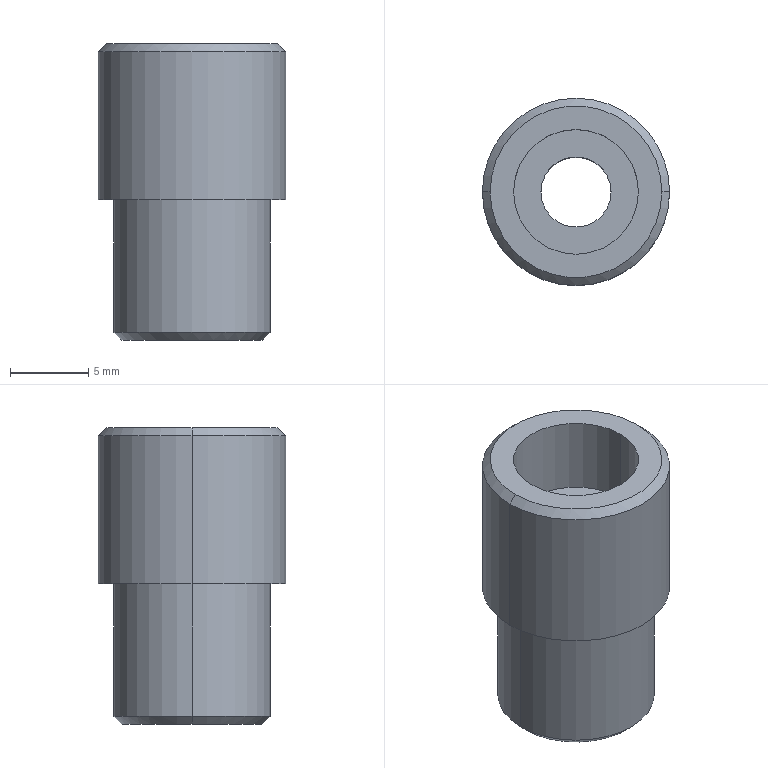Part | STEP file | 227H056246 Shaft_Default | 1 solid | 16 faces | box 12 x 12 x 19 mm | volume 1355 mm3 | cylinder 8 | cone 4 | plane 4 | commonest cylinder face diameters 4.5 x2 8 x2 10 x2 12 x2
STEP:
#1=CARTESIAN_POINT('',(0.,0.,0.));
#2=DIRECTION('',(0.,0.,1.));
#3=DIRECTION('',(1.,0.,0.));
#4=AXIS2_PLACEMENT_3D('',#1,#2,#3);
#5=CARTESIAN_POINT('',(-4.5,0.,-2.));
#6=VERTEX_POINT('',#5);
#7=CARTESIAN_POINT('',(4.5,0.,-2.));
#8=VERTEX_POINT('',#7);
#9=CARTESIAN_POINT('',(0.,0.,-2.));
#10=DIRECTION('',(0.,0.,-1.));
#11=DIRECTION('',(-1.,0.,0.));
#12=AXIS2_PLACEMENT_3D('',#9,#10,#11);
#13=CIRCLE('',#12,4.5);
#14=CARTESIAN_POINT('',(0.,0.,-2.));
#15=DIRECTION('',(0.,0.,1.));
#16=DIRECTION('',(1.,0.,0.));
#17=AXIS2_PLACEMENT_3D('',#14,#15,#16);
#18=CONICAL_SURFACE('',#17,4.5,0.7854);
#19=CARTESIAN_POINT('',(3.142,0.));
#20=DIRECTION('',(-1.,0.));
#21=VECTOR('',#20,1.);
#22=LINE('',#19,#21);
#23=(GEOMETRIC_REPRESENTATION_CONTEXT(2)PARAMETRIC_REPRESENTATION_CONTEXT()REPRESENTATION_CONTEXT('',''));
#24=DEFINITIONAL_REPRESENTATION('',(#22),#23);
#25=PCURVE('',#18,#24);
#26=CARTESIAN_POINT('',(0.,0.,-2.));
#27=DIRECTION('',(0.,0.,-1.));
#28=DIRECTION('',(-1.,0.,0.));
#29=AXIS2_PLACEMENT_3D('',#26,#27,#28);
#30=PLANE('',#29);
#31=CARTESIAN_POINT('',(0.,0.));
#32=DIRECTION('',(1.,0.));
#33=AXIS2_PLACEMENT_2D('',#31,#32);
#34=CIRCLE('',#33,4.5);
#35=(GEOMETRIC_REPRESENTATION_CONTEXT(2)PARAMETRIC_REPRESENTATION_CONTEXT()REPRESENTATION_CONTEXT('',''));
#36=DEFINITIONAL_REPRESENTATION('',(#34),#35);
#37=PCURVE('',#30,#36);
#38=SURFACE_CURVE('',#13,(#25,#37),.PCURVE_S1.);
#39=EDGE_CURVE('',#6,#8,#38,.T.);
#40=ORIENTED_EDGE('',*,*,#39,.F.);
#41=CARTESIAN_POINT('',(-5.,0.,-1.5));
#42=VERTEX_POINT('',#41);
#43=CARTESIAN_POINT('',(-4.5,0.,-2.));
#44=DIRECTION('',(-0.7071,0.,0.7071));
#45=VECTOR('',#44,1.);
#46=LINE('',#43,#45);
#47=CARTESIAN_POINT('',(3.142,0.));
#48=DIRECTION('',(0.,1.));
#49=VECTOR('',#48,1.);
#50=LINE('',#47,#49);
#51=(GEOMETRIC_REPRESENTATION_CONTEXT(2)PARAMETRIC_REPRESENTATION_CONTEXT()REPRESENTATION_CONTEXT('',''));
#52=DEFINITIONAL_REPRESENTATION('',(#50),#51);
#53=PCURVE('',#18,#52);
#54=CARTESIAN_POINT('',(0.,0.,-2.));
#55=DIRECTION('',(0.,0.,1.));
#56=DIRECTION('',(1.,0.,0.));
#57=AXIS2_PLACEMENT_3D('',#54,#55,#56);
#58=CONICAL_SURFACE('',#57,4.5,0.7854);
#59=CARTESIAN_POINT('',(3.142,0.));
#60=DIRECTION('',(0.,1.));
#61=VECTOR('',#60,1.);
#62=LINE('',#59,#61);
#63=(GEOMETRIC_REPRESENTATION_CONTEXT(2)PARAMETRIC_REPRESENTATION_CONTEXT()REPRESENTATION_CONTEXT('',''));
#64=DEFINITIONAL_REPRESENTATION('',(#62),#63);
#65=PCURVE('',#58,#64);
#66=SURFACE_CURVE('',#46,(#53,#65),.PCURVE_S1.);
#67=EDGE_CURVE('',#6,#42,#66,.T.);
#68=ORIENTED_EDGE('',*,*,#67,.T.);
#69=CARTESIAN_POINT('',(5.,0.,-1.5));
#70=VERTEX_POINT('',#69);
#71=CARTESIAN_POINT('',(0.,0.,-1.5));
#72=DIRECTION('',(0.,0.,1.));
#73=DIRECTION('',(-1.,0.,0.));
#74=AXIS2_PLACEMENT_3D('',#71,#72,#73);
#75=CIRCLE('',#74,5.);
#76=CARTESIAN_POINT('',(-3.142,0.5));
#77=DIRECTION('',(1.,0.));
#78=VECTOR('',#77,1.);
#79=LINE('',#76,#78);
#80=(GEOMETRIC_REPRESENTATION_CONTEXT(2)PARAMETRIC_REPRESENTATION_CONTEXT()REPRESENTATION_CONTEXT('',''));
#81=DEFINITIONAL_REPRESENTATION('',(#79),#80);
#82=PCURVE('',#18,#81);
#83=CARTESIAN_POINT('',(0.,0.,12.));
#84=DIRECTION('',(0.,0.,-1.));
#85=DIRECTION('',(-1.,0.,0.));
#86=AXIS2_PLACEMENT_3D('',#83,#84,#85);
#87=CYLINDRICAL_SURFACE('',#86,5.);
#88=CARTESIAN_POINT('',(6.283,13.5));
#89=DIRECTION('',(-1.,0.));
#90=VECTOR('',#89,1.);
#91=LINE('',#88,#90);
#92=(GEOMETRIC_REPRESENTATION_CONTEXT(2)PARAMETRIC_REPRESENTATION_CONTEXT()REPRESENTATION_CONTEXT('',''));
#93=DEFINITIONAL_REPRESENTATION('',(#91),#92);
#94=PCURVE('',#87,#93);
#95=SURFACE_CURVE('',#75,(#82,#94),.PCURVE_S1.);
#96=EDGE_CURVE('',#70,#42,#95,.T.);
#97=ORIENTED_EDGE('',*,*,#96,.F.);
#98=CARTESIAN_POINT('',(4.5,0.,-2.));
#99=DIRECTION('',(0.7071,0.,0.7071));
#100=VECTOR('',#99,1.);
#101=LINE('',#98,#100);
#102=CARTESIAN_POINT('',(0.,0.));
#103=DIRECTION('',(0.,1.));
#104=VECTOR('',#103,1.);
#105=LINE('',#102,#104);
#106=(GEOMETRIC_REPRESENTATION_CONTEXT(2)PARAMETRIC_REPRESENTATION_CONTEXT()REPRESENTATION_CONTEXT('',''));
#107=DEFINITIONAL_REPRESENTATION('',(#105),#106);
#108=PCURVE('',#18,#107);
#109=CARTESIAN_POINT('',(6.283,0.));
#110=DIRECTION('',(0.,1.));
#111=VECTOR('',#110,1.);
#112=LINE('',#109,#111);
#113=(GEOMETRIC_REPRESENTATION_CONTEXT(2)PARAMETRIC_REPRESENTATION_CONTEXT()REPRESENTATION_CONTEXT('',''));
#114=DEFINITIONAL_REPRESENTATION('',(#112),#113);
#115=PCURVE('',#58,#114);
#116=SURFACE_CURVE('',#101,(#108,#115),.PCURVE_S1.);
#117=EDGE_CURVE('',#8,#70,#116,.T.);
#118=ORIENTED_EDGE('',*,*,#117,.F.);
#119=EDGE_LOOP('',(#40,#68,#97,#118));
#120=FACE_BOUND('',#119,.T.);
#121=ADVANCED_FACE('',(#120),#18,.T.);
#122=CARTESIAN_POINT('',(5.5,0.,17.));
#123=VERTEX_POINT('',#122);
#124=CARTESIAN_POINT('',(-5.5,0.,17.));
#125=VERTEX_POINT('',#124);
#126=CARTESIAN_POINT('',(0.,0.,17.));
#127=DIRECTION('',(0.,0.,1.));
#128=DIRECTION('',(1.,0.,0.));
#129=AXIS2_PLACEMENT_3D('',#126,#127,#128);
#130=CIRCLE('',#129,5.5);
#131=CARTESIAN_POINT('',(0.,0.,17.));
#132=DIRECTION('',(0.,0.,-1.));
#133=DIRECTION('',(-1.,0.,0.));
#134=AXIS2_PLACEMENT_3D('',#131,#132,#133);
#135=CONICAL_SURFACE('',#134,5.5,0.7854);
#136=CARTESIAN_POINT('',(3.142,0.));
#137=DIRECTION('',(-1.,0.));
#138=VECTOR('',#137,1.);
#139=LINE('',#136,#138);
#140=(GEOMETRIC_REPRESENTATION_CONTEXT(2)PARAMETRIC_REPRESENTATION_CONTEXT()REPRESENTATION_CONTEXT('',''));
#141=DEFINITIONAL_REPRESENTATION('',(#139),#140);
#142=PCURVE('',#135,#141);
#143=CARTESIAN_POINT('',(0.,0.,17.));
#144=DIRECTION('',(0.,0.,1.));
#145=DIRECTION('',(1.,0.,0.));
#146=AXIS2_PLACEMENT_3D('',#143,#144,#145);
#147=PLANE('',#146);
#148=CARTESIAN_POINT('',(0.,0.));
#149=DIRECTION('',(1.,0.));
#150=AXIS2_PLACEMENT_2D('',#148,#149);
#151=CIRCLE('',#150,5.5);
#152=(GEOMETRIC_REPRESENTATION_CONTEXT(2)PARAMETRIC_REPRESENTATION_CONTEXT()REPRESENTATION_CONTEXT('',''));
#153=DEFINITIONAL_REPRESENTATION('',(#151),#152);
#154=PCURVE('',#147,#153);
#155=SURFACE_CURVE('',#130,(#142,#154),.PCURVE_S1.);
#156=EDGE_CURVE('',#123,#125,#155,.T.);
#157=ORIENTED_EDGE('',*,*,#156,.F.);
#158=CARTESIAN_POINT('',(6.,0.,16.5));
#159=VERTEX_POINT('',#158);
#160=CARTESIAN_POINT('',(5.5,0.,17.));
#161=DIRECTION('',(0.7071,0.,-0.7071));
#162=VECTOR('',#161,1.);
#163=LINE('',#160,#162);
#164=CARTESIAN_POINT('',(3.142,0.));
#165=DIRECTION('',(0.,1.));
#166=VECTOR('',#165,1.);
#167=LINE('',#164,#166);
#168=(GEOMETRIC_REPRESENTATION_CONTEXT(2)PARAMETRIC_REPRESENTATION_CONTEXT()REPRESENTATION_CONTEXT('',''));
#169=DEFINITIONAL_REPRESENTATION('',(#167),#168);
#170=PCURVE('',#135,#169);
#171=CARTESIAN_POINT('',(0.,0.,17.));
#172=DIRECTION('',(0.,0.,-1.));
#173=DIRECTION('',(-1.,0.,0.));
#174=AXIS2_PLACEMENT_3D('',#171,#172,#173);
#175=CONICAL_SURFACE('',#174,5.5,0.7854);
#176=CARTESIAN_POINT('',(3.142,0.));
#177=DIRECTION('',(0.,1.));
#178=VECTOR('',#177,1.);
#179=LINE('',#176,#178);
#180=(GEOMETRIC_REPRESENTATION_CONTEXT(2)PARAMETRIC_REPRESENTATION_CONTEXT()REPRESENTATION_CONTEXT('',''));
#181=DEFINITIONAL_REPRESENTATION('',(#179),#180);
#182=PCURVE('',#175,#181);
#183=SURFACE_CURVE('',#163,(#170,#182),.PCURVE_S1.);
#184=EDGE_CURVE('',#123,#159,#183,.T.);
#185=ORIENTED_EDGE('',*,*,#184,.T.);
#186=CARTESIAN_POINT('',(-6.,0.,16.5));
#187=VERTEX_POINT('',#186);
#188=CARTESIAN_POINT('',(0.,0.,16.5));
#189=DIRECTION('',(0.,0.,-1.));
#190=DIRECTION('',(1.,0.,0.));
#191=AXIS2_PLACEMENT_3D('',#188,#189,#190);
#192=CIRCLE('',#191,6.);
#193=CARTESIAN_POINT('',(-3.142,0.5));
#194=DIRECTION('',(1.,0.));
#195=VECTOR('',#194,1.);
#196=LINE('',#193,#195);
#197=(GEOMETRIC_REPRESENTATION_CONTEXT(2)PARAMETRIC_REPRESENTATION_CONTEXT()REPRESENTATION_CONTEXT('',''));
#198=DEFINITIONAL_REPRESENTATION('',(#196),#197);
#199=PCURVE('',#135,#198);
#200=CARTESIAN_POINT('',(0.,0.,17.));
#201=DIRECTION('',(0.,0.,-1.));
#202=DIRECTION('',(-1.,0.,0.));
#203=AXIS2_PLACEMENT_3D('',#200,#201,#202);
#204=CYLINDRICAL_SURFACE('',#203,6.);
#205=CARTESIAN_POINT('',(-3.142,0.5));
#206=DIRECTION('',(1.,0.));
#207=VECTOR('',#206,1.);
#208=LINE('',#205,#207);
#209=(GEOMETRIC_REPRESENTATION_CONTEXT(2)PARAMETRIC_REPRESENTATION_CONTEXT()REPRESENTATION_CONTEXT('',''));
#210=DEFINITIONAL_REPRESENTATION('',(#208),#209);
#211=PCURVE('',#204,#210);
#212=SURFACE_CURVE('',#192,(#199,#211),.PCURVE_S1.);
#213=EDGE_CURVE('',#187,#159,#212,.T.);
#214=ORIENTED_EDGE('',*,*,#213,.F.);
#215=CARTESIAN_POINT('',(-5.5,0.,17.));
#216=DIRECTION('',(-0.7071,0.,-0.7071));
#217=VECTOR('',#216,1.);
#218=LINE('',#215,#217);
#219=CARTESIAN_POINT('',(0.,0.));
#220=DIRECTION('',(0.,1.));
#221=VECTOR('',#220,1.);
#222=LINE('',#219,#221);
#223=(GEOMETRIC_REPRESENTATION_CONTEXT(2)PARAMETRIC_REPRESENTATION_CONTEXT()REPRESENTATION_CONTEXT('',''));
#224=DEFINITIONAL_REPRESENTATION('',(#222),#223);
#225=PCURVE('',#135,#224);
#226=CARTESIAN_POINT('',(6.283,0.));
#227=DIRECTION('',(0.,1.));
#228=VECTOR('',#227,1.);
#229=LINE('',#226,#228);
#230=(GEOMETRIC_REPRESENTATION_CONTEXT(2)PARAMETRIC_REPRESENTATION_CONTEXT()REPRESENTATION_CONTEXT('',''));
#231=DEFINITIONAL_REPRESENTATION('',(#229),#230);
#232=PCURVE('',#175,#231);
#233=SURFACE_CURVE('',#218,(#225,#232),.PCURVE_S1.);
#234=EDGE_CURVE('',#125,#187,#233,.T.);
#235=ORIENTED_EDGE('',*,*,#234,.F.);
#236=EDGE_LOOP('',(#157,#185,#214,#235));
#237=FACE_BOUND('',#236,.T.);
#238=ADVANCED_FACE('',(#237),#135,.T.);
#239=CARTESIAN_POINT('',(4.,0.,12.));
#240=VERTEX_POINT('',#239);
#241=CARTESIAN_POINT('',(4.,0.,17.));
#242=VERTEX_POINT('',#241);
#243=CARTESIAN_POINT('',(4.,0.,17.));
#244=DIRECTION('',(0.,0.,1.));
#245=VECTOR('',#244,1.);
#246=LINE('',#243,#245);
#247=CARTESIAN_POINT('',(0.,0.,17.));
#248=DIRECTION('',(0.,0.,1.));
#249=DIRECTION('',(1.,0.,0.));
#250=AXIS2_PLACEMENT_3D('',#247,#248,#249);
#251=CYLINDRICAL_SURFACE('',#250,4.);
#252=CARTESIAN_POINT('',(6.283,0.));
#253=DIRECTION('',(0.,1.));
#254=VECTOR('',#253,1.);
#255=LINE('',#252,#254);
#256=(GEOMETRIC_REPRESENTATION_CONTEXT(2)PARAMETRIC_REPRESENTATION_CONTEXT()REPRESENTATION_CONTEXT('',''));
#257=DEFINITIONAL_REPRESENTATION('',(#255),#256);
#258=PCURVE('',#251,#257);
#259=CARTESIAN_POINT('',(0.,0.,17.));
#260=DIRECTION('',(0.,0.,1.));
#261=DIRECTION('',(1.,0.,0.));
#262=AXIS2_PLACEMENT_3D('',#259,#260,#261);
#263=CYLINDRICAL_SURFACE('',#262,4.);
#264=CARTESIAN_POINT('',(0.,0.));
#265=DIRECTION('',(0.,1.));
#266=VECTOR('',#265,1.);
#267=LINE('',#264,#266);
#268=(GEOMETRIC_REPRESENTATION_CONTEXT(2)PARAMETRIC_REPRESENTATION_CONTEXT()REPRESENTATION_CONTEXT('',''));
#269=DEFINITIONAL_REPRESENTATION('',(#267),#268);
#270=PCURVE('',#263,#269);
#271=SURFACE_CURVE('',#246,(#258,#270),.PCURVE_S1.);
#272=EDGE_CURVE('',#240,#242,#271,.T.);
#273=ORIENTED_EDGE('',*,*,#272,.T.);
#274=CARTESIAN_POINT('',(-4.,0.,17.));
#275=VERTEX_POINT('',#274);
#276=CARTESIAN_POINT('',(0.,0.,17.));
#277=DIRECTION('',(0.,0.,1.));
#278=DIRECTION('',(1.,0.,0.));
#279=AXIS2_PLACEMENT_3D('',#276,#277,#278);
#280=CIRCLE('',#279,4.);
#281=CARTESIAN_POINT('',(0.,0.));
#282=DIRECTION('',(1.,0.));
#283=VECTOR('',#282,1.);
#284=LINE('',#281,#283);
#285=(GEOMETRIC_REPRESENTATION_CONTEXT(2)PARAMETRIC_REPRESENTATION_CONTEXT()REPRESENTATION_CONTEXT('',''));
#286=DEFINITIONAL_REPRESENTATION('',(#284),#285);
#287=PCURVE('',#251,#286);
#288=CARTESIAN_POINT('',(0.,0.));
#289=DIRECTION('',(1.,0.));
#290=AXIS2_PLACEMENT_2D('',#288,#289);
#291=CIRCLE('',#290,4.);
#292=(GEOMETRIC_REPRESENTATION_CONTEXT(2)PARAMETRIC_REPRESENTATION_CONTEXT()REPRESENTATION_CONTEXT('',''));
#293=DEFINITIONAL_REPRESENTATION('',(#291),#292);
#294=PCURVE('',#147,#293);
#295=SURFACE_CURVE('',#280,(#287,#294),.PCURVE_S1.);
#296=EDGE_CURVE('',#275,#242,#295,.T.);
#297=ORIENTED_EDGE('',*,*,#296,.F.);
#298=CARTESIAN_POINT('',(-4.,0.,12.));
#299=VERTEX_POINT('',#298);
#300=CARTESIAN_POINT('',(-4.,0.,17.));
#301=DIRECTION('',(0.,0.,1.));
#302=VECTOR('',#301,1.);
#303=LINE('',#300,#302);
#304=CARTESIAN_POINT('',(3.142,0.));
#305=DIRECTION('',(0.,1.));
#306=VECTOR('',#305,1.);
#307=LINE('',#304,#306);
#308=(GEOMETRIC_REPRESENTATION_CONTEXT(2)PARAMETRIC_REPRESENTATION_CONTEXT()REPRESENTATION_CONTEXT('',''));
#309=DEFINITIONAL_REPRESENTATION('',(#307),#308);
#310=PCURVE('',#251,#309);
#311=CARTESIAN_POINT('',(3.142,0.));
#312=DIRECTION('',(0.,1.));
#313=VECTOR('',#312,1.);
#314=LINE('',#311,#313);
#315=(GEOMETRIC_REPRESENTATION_CONTEXT(2)PARAMETRIC_REPRESENTATION_CONTEXT()REPRESENTATION_CONTEXT('',''));
#316=DEFINITIONAL_REPRESENTATION('',(#314),#315);
#317=PCURVE('',#263,#316);
#318=SURFACE_CURVE('',#303,(#310,#317),.PCURVE_S1.);
#319=EDGE_CURVE('',#299,#275,#318,.T.);
#320=ORIENTED_EDGE('',*,*,#319,.F.);
#321=CARTESIAN_POINT('',(0.,0.,12.));
#322=DIRECTION('',(0.,0.,1.));
#323=DIRECTION('',(1.,0.,0.));
#324=AXIS2_PLACEMENT_3D('',#321,#322,#323);
#325=CIRCLE('',#324,4.);
#326=CARTESIAN_POINT('',(0.,-5.));
#327=DIRECTION('',(1.,0.));
#328=VECTOR('',#327,1.);
#329=LINE('',#326,#328);
#330=(GEOMETRIC_REPRESENTATION_CONTEXT(2)PARAMETRIC_REPRESENTATION_CONTEXT()REPRESENTATION_CONTEXT('',''));
#331=DEFINITIONAL_REPRESENTATION('',(#329),#330);
#332=PCURVE('',#251,#331);
#333=CARTESIAN_POINT('',(2.25,0.,12.));
#334=DIRECTION('',(0.,0.,-1.));
#335=DIRECTION('',(-1.,0.,0.));
#336=AXIS2_PLACEMENT_3D('',#333,#334,#335);
#337=PLANE('',#336);
#338=CARTESIAN_POINT('',(-1.75,0.));
#339=CARTESIAN_POINT('',(-1.75,6.928));
#340=CARTESIAN_POINT('',(4.25,3.464));
#341=CARTESIAN_POINT('',(10.25,0.));
#342=CARTESIAN_POINT('',(4.25,-3.464));
#343=CARTESIAN_POINT('',(-1.75,-6.928));
#344=CARTESIAN_POINT('',(-1.75,0.));
#345=(BOUNDED_CURVE()B_SPLINE_CURVE(2,(#338,#339,#340,#341,#342,#343,#344),.UNSPECIFIED.,.T.,.F.)B_SPLINE_CURVE_WITH_KNOTS((1,2,2,2,2,1),(-2.094,0.,2.094,4.189,6.283,8.378),.UNSPECIFIED.)CURVE()GEOMETRIC_REPRESENTATION_ITEM()RATIONAL_B_SPLINE_CURVE((1.,0.5,1.,0.5,1.,0.5,1.))REPRESENTATION_ITEM(''));
#346=(GEOMETRIC_REPRESENTATION_CONTEXT(2)PARAMETRIC_REPRESENTATION_CONTEXT()REPRESENTATION_CONTEXT('',''));
#347=DEFINITIONAL_REPRESENTATION('',(#345),#346);
#348=PCURVE('',#337,#347);
#349=SURFACE_CURVE('',#325,(#332,#348),.PCURVE_S1.);
#350=EDGE_CURVE('',#299,#240,#349,.T.);
#351=ORIENTED_EDGE('',*,*,#350,.T.);
#352=EDGE_LOOP('',(#273,#297,#320,#351));
#353=FACE_BOUND('',#352,.F.);
#354=ADVANCED_FACE('',(#353),#251,.F.);
#355=CARTESIAN_POINT('',(2.25,0.,-2.));
#356=VERTEX_POINT('',#355);
#357=CARTESIAN_POINT('',(2.25,0.,12.));
#358=VERTEX_POINT('',#357);
#359=CARTESIAN_POINT('',(2.25,0.,17.));
#360=DIRECTION('',(0.,0.,1.));
#361=VECTOR('',#360,1.);
#362=LINE('',#359,#361);
#363=CARTESIAN_POINT('',(0.,0.,17.));
#364=DIRECTION('',(0.,0.,1.));
#365=DIRECTION('',(1.,0.,0.));
#366=AXIS2_PLACEMENT_3D('',#363,#364,#365);
#367=CYLINDRICAL_SURFACE('',#366,2.25);
#368=CARTESIAN_POINT('',(6.283,0.));
#369=DIRECTION('',(0.,1.));
#370=VECTOR('',#369,1.);
#371=LINE('',#368,#370);
#372=(GEOMETRIC_REPRESENTATION_CONTEXT(2)PARAMETRIC_REPRESENTATION_CONTEXT()REPRESENTATION_CONTEXT('',''));
#373=DEFINITIONAL_REPRESENTATION('',(#371),#372);
#374=PCURVE('',#367,#373);
#375=CARTESIAN_POINT('',(0.,0.,17.));
#376=DIRECTION('',(0.,0.,1.));
#377=DIRECTION('',(1.,0.,0.));
#378=AXIS2_PLACEMENT_3D('',#375,#376,#377);
#379=CYLINDRICAL_SURFACE('',#378,2.25);
#380=CARTESIAN_POINT('',(0.,0.));
#381=DIRECTION('',(0.,1.));
#382=VECTOR('',#381,1.);
#383=LINE('',#380,#382);
#384=(GEOMETRIC_REPRESENTATION_CONTEXT(2)PARAMETRIC_REPRESENTATION_CONTEXT()REPRESENTATION_CONTEXT('',''));
#385=DEFINITIONAL_REPRESENTATION('',(#383),#384);
#386=PCURVE('',#379,#385);
#387=SURFACE_CURVE('',#362,(#374,#386),.PCURVE_S1.);
#388=EDGE_CURVE('',#356,#358,#387,.T.);
#389=ORIENTED_EDGE('',*,*,#388,.T.);
#390=CARTESIAN_POINT('',(-2.25,0.,12.));
#391=VERTEX_POINT('',#390);
#392=CARTESIAN_POINT('',(0.,0.,12.));
#393=DIRECTION('',(0.,0.,1.));
#394=DIRECTION('',(1.,0.,0.));
#395=AXIS2_PLACEMENT_3D('',#392,#393,#394);
#396=CIRCLE('',#395,2.25);
#397=CARTESIAN_POINT('',(0.,-5.));
#398=DIRECTION('',(1.,0.));
#399=VECTOR('',#398,1.);
#400=LINE('',#397,#399);
#401=(GEOMETRIC_REPRESENTATION_CONTEXT(2)PARAMETRIC_REPRESENTATION_CONTEXT()REPRESENTATION_CONTEXT('',''));
#402=DEFINITIONAL_REPRESENTATION('',(#400),#401);
#403=PCURVE('',#367,#402);
#404=CARTESIAN_POINT('',(0.,0.));
#405=CARTESIAN_POINT('',(0.,3.897));
#406=CARTESIAN_POINT('',(3.375,1.949));
#407=CARTESIAN_POINT('',(6.75,0.));
#408=CARTESIAN_POINT('',(3.375,-1.949));
#409=CARTESIAN_POINT('',(0.,-3.897));
#410=CARTESIAN_POINT('',(0.,0.));
#411=(BOUNDED_CURVE()B_SPLINE_CURVE(2,(#404,#405,#406,#407,#408,#409,#410),.UNSPECIFIED.,.T.,.F.)B_SPLINE_CURVE_WITH_KNOTS((1,2,2,2,2,1),(-2.094,0.,2.094,4.189,6.283,8.378),.UNSPECIFIED.)CURVE()GEOMETRIC_REPRESENTATION_ITEM()RATIONAL_B_SPLINE_CURVE((1.,0.5,1.,0.5,1.,0.5,1.))REPRESENTATION_ITEM(''));
#412=(GEOMETRIC_REPRESENTATION_CONTEXT(2)PARAMETRIC_REPRESENTATION_CONTEXT()REPRESENTATION_CONTEXT('',''));
#413=DEFINITIONAL_REPRESENTATION('',(#411),#412);
#414=PCURVE('',#337,#413);
#415=SURFACE_CURVE('',#396,(#403,#414),.PCURVE_S1.);
#416=EDGE_CURVE('',#391,#358,#415,.T.);
#417=ORIENTED_EDGE('',*,*,#416,.F.);
#418=CARTESIAN_POINT('',(-2.25,0.,-2.));
#419=VERTEX_POINT('',#418);
#420=CARTESIAN_POINT('',(-2.25,0.,17.));
#421=DIRECTION('',(0.,0.,1.));
#422=VECTOR('',#421,1.);
#423=LINE('',#420,#422);
#424=CARTESIAN_POINT('',(3.142,0.));
#425=DIRECTION('',(0.,1.));
#426=VECTOR('',#425,1.);
#427=LINE('',#424,#426);
#428=(GEOMETRIC_REPRESENTATION_CONTEXT(2)PARAMETRIC_REPRESENTATION_CONTEXT()REPRESENTATION_CONTEXT('',''));
#429=DEFINITIONAL_REPRESENTATION('',(#427),#428);
#430=PCURVE('',#367,#429);
#431=CARTESIAN_POINT('',(3.142,0.));
#432=DIRECTION('',(0.,1.));
#433=VECTOR('',#432,1.);
#434=LINE('',#431,#433);
#435=(GEOMETRIC_REPRESENTATION_CONTEXT(2)PARAMETRIC_REPRESENTATION_CONTEXT()REPRESENTATION_CONTEXT('',''));
#436=DEFINITIONAL_REPRESENTATION('',(#434),#435);
#437=PCURVE('',#379,#436);
#438=SURFACE_CURVE('',#423,(#430,#437),.PCURVE_S1.);
#439=EDGE_CURVE('',#419,#391,#438,.T.);
#440=ORIENTED_EDGE('',*,*,#439,.F.);
#441=CARTESIAN_POINT('',(0.,0.,-2.));
#442=DIRECTION('',(0.,0.,1.));
#443=DIRECTION('',(1.,0.,0.));
#444=AXIS2_PLACEMENT_3D('',#441,#442,#443);
#445=CIRCLE('',#444,2.25);
#446=CARTESIAN_POINT('',(0.,-19.));
#447=DIRECTION('',(1.,0.));
#448=VECTOR('',#447,1.);
#449=LINE('',#446,#448);
#450=(GEOMETRIC_REPRESENTATION_CONTEXT(2)PARAMETRIC_REPRESENTATION_CONTEXT()REPRESENTATION_CONTEXT('',''));
#451=DEFINITIONAL_REPRESENTATION('',(#449),#450);
#452=PCURVE('',#367,#451);
#453=CARTESIAN_POINT('',(-2.25,0.));
#454=CARTESIAN_POINT('',(-2.25,3.897));
#455=CARTESIAN_POINT('',(1.125,1.949));
#456=CARTESIAN_POINT('',(4.5,0.));
#457=CARTESIAN_POINT('',(1.125,-1.949));
#458=CARTESIAN_POINT('',(-2.25,-3.897));
#459=CARTESIAN_POINT('',(-2.25,0.));
#460=(BOUNDED_CURVE()B_SPLINE_CURVE(2,(#453,#454,#455,#456,#457,#458,#459),.UNSPECIFIED.,.T.,.F.)B_SPLINE_CURVE_WITH_KNOTS((1,2,2,2,2,1),(-2.094,0.,2.094,4.189,6.283,8.378),.UNSPECIFIED.)CURVE()GEOMETRIC_REPRESENTATION_ITEM()RATIONAL_B_SPLINE_CURVE((1.,0.5,1.,0.5,1.,0.5,1.))REPRESENTATION_ITEM(''));
#461=(GEOMETRIC_REPRESENTATION_CONTEXT(2)PARAMETRIC_REPRESENTATION_CONTEXT()REPRESENTATION_CONTEXT('',''));
#462=DEFINITIONAL_REPRESENTATION('',(#460),#461);
#463=PCURVE('',#30,#462);
#464=SURFACE_CURVE('',#445,(#452,#463),.PCURVE_S1.);
#465=EDGE_CURVE('',#419,#356,#464,.T.);
#466=ORIENTED_EDGE('',*,*,#465,.T.);
#467=EDGE_LOOP('',(#389,#417,#440,#466));
#468=FACE_BOUND('',#467,.F.);
#469=ADVANCED_FACE('',(#468),#367,.F.);
#470=ORIENTED_EDGE('',*,*,#213,.T.);
#471=CARTESIAN_POINT('',(6.,0.,7.));
#472=VERTEX_POINT('',#471);
#473=CARTESIAN_POINT('',(6.,0.,17.));
#474=DIRECTION('',(0.,0.,-1.));
#475=VECTOR('',#474,1.);
#476=LINE('',#473,#475);
#477=CARTESIAN_POINT('',(3.142,0.));
#478=DIRECTION('',(0.,1.));
#479=VECTOR('',#478,1.);
#480=LINE('',#477,#479);
#481=(GEOMETRIC_REPRESENTATION_CONTEXT(2)PARAMETRIC_REPRESENTATION_CONTEXT()REPRESENTATION_CONTEXT('',''));
#482=DEFINITIONAL_REPRESENTATION('',(#480),#481);
#483=PCURVE('',#204,#482);
#484=CARTESIAN_POINT('',(0.,0.,17.));
#485=DIRECTION('',(0.,0.,-1.));
#486=DIRECTION('',(-1.,0.,0.));
#487=AXIS2_PLACEMENT_3D('',#484,#485,#486);
#488=CYLINDRICAL_SURFACE('',#487,6.);
#489=CARTESIAN_POINT('',(3.142,0.));
#490=DIRECTION('',(0.,1.));
#491=VECTOR('',#490,1.);
#492=LINE('',#489,#491);
#493=(GEOMETRIC_REPRESENTATION_CONTEXT(2)PARAMETRIC_REPRESENTATION_CONTEXT()REPRESENTATION_CONTEXT('',''));
#494=DEFINITIONAL_REPRESENTATION('',(#492),#493);
#495=PCURVE('',#488,#494);
#496=SURFACE_CURVE('',#476,(#483,#495),.PCURVE_S1.);
#497=EDGE_CURVE('',#159,#472,#496,.T.);
#498=ORIENTED_EDGE('',*,*,#497,.T.);
#499=CARTESIAN_POINT('',(-6.,0.,7.));
#500=VERTEX_POINT('',#499);
#501=CARTESIAN_POINT('',(0.,0.,7.));
#502=DIRECTION('',(0.,0.,1.));
#503=DIRECTION('',(1.,0.,0.));
#504=AXIS2_PLACEMENT_3D('',#501,#502,#503);
#505=CIRCLE('',#504,6.);
#506=CARTESIAN_POINT('',(3.142,10.));
#507=DIRECTION('',(-1.,0.));
#508=VECTOR('',#507,1.);
#509=LINE('',#506,#508);
#510=(GEOMETRIC_REPRESENTATION_CONTEXT(2)PARAMETRIC_REPRESENTATION_CONTEXT()REPRESENTATION_CONTEXT('',''));
#511=DEFINITIONAL_REPRESENTATION('',(#509),#510);
#512=PCURVE('',#204,#511);
#513=CARTESIAN_POINT('',(0.,0.,7.));
#514=DIRECTION('',(0.,0.,1.));
#515=DIRECTION('',(1.,0.,0.));
#516=AXIS2_PLACEMENT_3D('',#513,#514,#515);
#517=PLANE('',#516);
#518=CARTESIAN_POINT('',(0.,0.));
#519=DIRECTION('',(1.,0.));
#520=AXIS2_PLACEMENT_2D('',#518,#519);
#521=CIRCLE('',#520,6.);
#522=(GEOMETRIC_REPRESENTATION_CONTEXT(2)PARAMETRIC_REPRESENTATION_CONTEXT()REPRESENTATION_CONTEXT('',''));
#523=DEFINITIONAL_REPRESENTATION('',(#521),#522);
#524=PCURVE('',#517,#523);
#525=SURFACE_CURVE('',#505,(#512,#524),.PCURVE_S1.);
#526=EDGE_CURVE('',#472,#500,#525,.T.);
#527=ORIENTED_EDGE('',*,*,#526,.T.);
#528=CARTESIAN_POINT('',(-6.,0.,17.));
#529=DIRECTION('',(0.,0.,-1.));
#530=VECTOR('',#529,1.);
#531=LINE('',#528,#530);
#532=CARTESIAN_POINT('',(0.,0.));
#533=DIRECTION('',(0.,1.));
#534=VECTOR('',#533,1.);
#535=LINE('',#532,#534);
#536=(GEOMETRIC_REPRESENTATION_CONTEXT(2)PARAMETRIC_REPRESENTATION_CONTEXT()REPRESENTATION_CONTEXT('',''));
#537=DEFINITIONAL_REPRESENTATION('',(#535),#536);
#538=PCURVE('',#204,#537);
#539=CARTESIAN_POINT('',(6.283,0.));
#540=DIRECTION('',(0.,1.));
#541=VECTOR('',#540,1.);
#542=LINE('',#539,#541);
#543=(GEOMETRIC_REPRESENTATION_CONTEXT(2)PARAMETRIC_REPRESENTATION_CONTEXT()REPRESENTATION_CONTEXT('',''));
#544=DEFINITIONAL_REPRESENTATION('',(#542),#543);
#545=PCURVE('',#488,#544);
#546=SURFACE_CURVE('',#531,(#538,#545),.PCURVE_S1.);
#547=EDGE_CURVE('',#187,#500,#546,.T.);
#548=ORIENTED_EDGE('',*,*,#547,.F.);
#549=EDGE_LOOP('',(#470,#498,#527,#548));
#550=FACE_BOUND('',#549,.T.);
#551=ADVANCED_FACE('',(#550),#204,.T.);
#552=CARTESIAN_POINT('',(5.,0.,7.));
#553=VERTEX_POINT('',#552);
#554=CARTESIAN_POINT('',(-5.,0.,7.));
#555=VERTEX_POINT('',#554);
#556=CARTESIAN_POINT('',(0.,0.,7.));
#557=DIRECTION('',(0.,0.,1.));
#558=DIRECTION('',(1.,0.,0.));
#559=AXIS2_PLACEMENT_3D('',#556,#557,#558);
#560=CIRCLE('',#559,5.);
#561=CARTESIAN_POINT('',(3.142,5.));
#562=DIRECTION('',(-1.,0.));
#563=VECTOR('',#562,1.);
#564=LINE('',#561,#563);
#565=(GEOMETRIC_REPRESENTATION_CONTEXT(2)PARAMETRIC_REPRESENTATION_CONTEXT()REPRESENTATION_CONTEXT('',''));
#566=DEFINITIONAL_REPRESENTATION('',(#564),#565);
#567=PCURVE('',#87,#566);
#568=CARTESIAN_POINT('',(0.,0.));
#569=DIRECTION('',(1.,0.));
#570=AXIS2_PLACEMENT_2D('',#568,#569);
#571=CIRCLE('',#570,5.);
#572=(GEOMETRIC_REPRESENTATION_CONTEXT(2)PARAMETRIC_REPRESENTATION_CONTEXT()REPRESENTATION_CONTEXT('',''));
#573=DEFINITIONAL_REPRESENTATION('',(#571),#572);
#574=PCURVE('',#517,#573);
#575=SURFACE_CURVE('',#560,(#567,#574),.PCURVE_S1.);
#576=EDGE_CURVE('',#553,#555,#575,.T.);
#577=ORIENTED_EDGE('',*,*,#576,.F.);
#578=CARTESIAN_POINT('',(5.,0.,12.));
#579=DIRECTION('',(0.,0.,-1.));
#580=VECTOR('',#579,1.);
#581=LINE('',#578,#580);
#582=CARTESIAN_POINT('',(3.142,0.));
#583=DIRECTION('',(0.,1.));
#584=VECTOR('',#583,1.);
#585=LINE('',#582,#584);
#586=(GEOMETRIC_REPRESENTATION_CONTEXT(2)PARAMETRIC_REPRESENTATION_CONTEXT()REPRESENTATION_CONTEXT('',''));
#587=DEFINITIONAL_REPRESENTATION('',(#585),#586);
#588=PCURVE('',#87,#587);
#589=CARTESIAN_POINT('',(0.,0.,12.));
#590=DIRECTION('',(0.,0.,-1.));
#591=DIRECTION('',(-1.,0.,0.));
#592=AXIS2_PLACEMENT_3D('',#589,#590,#591);
#593=CYLINDRICAL_SURFACE('',#592,5.);
#594=CARTESIAN_POINT('',(3.142,0.));
#595=DIRECTION('',(0.,1.));
#596=VECTOR('',#595,1.);
#597=LINE('',#594,#596);
#598=(GEOMETRIC_REPRESENTATION_CONTEXT(2)PARAMETRIC_REPRESENTATION_CONTEXT()REPRESENTATION_CONTEXT('',''));
#599=DEFINITIONAL_REPRESENTATION('',(#597),#598);
#600=PCURVE('',#593,#599);
#601=SURFACE_CURVE('',#581,(#588,#600),.PCURVE_S1.);
#602=EDGE_CURVE('',#553,#70,#601,.T.);
#603=ORIENTED_EDGE('',*,*,#602,.T.);
#604=ORIENTED_EDGE('',*,*,#96,.T.);
#605=CARTESIAN_POINT('',(-5.,0.,12.));
#606=DIRECTION('',(0.,0.,-1.));
#607=VECTOR('',#606,1.);
#608=LINE('',#605,#607);
#609=CARTESIAN_POINT('',(0.,0.));
#610=DIRECTION('',(0.,1.));
#611=VECTOR('',#610,1.);
#612=LINE('',#609,#611);
#613=(GEOMETRIC_REPRESENTATION_CONTEXT(2)PARAMETRIC_REPRESENTATION_CONTEXT()REPRESENTATION_CONTEXT('',''));
#614=DEFINITIONAL_REPRESENTATION('',(#612),#613);
#615=PCURVE('',#87,#614);
#616=CARTESIAN_POINT('',(6.283,0.));
#617=DIRECTION('',(0.,1.));
#618=VECTOR('',#617,1.);
#619=LINE('',#616,#618);
#620=(GEOMETRIC_REPRESENTATION_CONTEXT(2)PARAMETRIC_REPRESENTATION_CONTEXT()REPRESENTATION_CONTEXT('',''));
#621=DEFINITIONAL_REPRESENTATION('',(#619),#620);
#622=PCURVE('',#593,#621);
#623=SURFACE_CURVE('',#608,(#615,#622),.PCURVE_S1.);
#624=EDGE_CURVE('',#555,#42,#623,.T.);
#625=ORIENTED_EDGE('',*,*,#624,.F.);
#626=EDGE_LOOP('',(#577,#603,#604,#625));
#627=FACE_BOUND('',#626,.T.);
#628=ADVANCED_FACE('',(#627),#87,.T.);
#629=ORIENTED_EDGE('',*,*,#602,.F.);
#630=CARTESIAN_POINT('',(0.,0.,7.));
#631=DIRECTION('',(0.,0.,1.));
#632=DIRECTION('',(1.,0.,0.));
#633=AXIS2_PLACEMENT_3D('',#630,#631,#632);
#634=CIRCLE('',#633,5.);
#635=CARTESIAN_POINT('',(9.425,5.));
#636=DIRECTION('',(-1.,0.));
#637=VECTOR('',#636,1.);
#638=LINE('',#635,#637);
#639=(GEOMETRIC_REPRESENTATION_CONTEXT(2)PARAMETRIC_REPRESENTATION_CONTEXT()REPRESENTATION_CONTEXT('',''));
#640=DEFINITIONAL_REPRESENTATION('',(#638),#639);
#641=PCURVE('',#593,#640);
#642=CARTESIAN_POINT('',(0.,0.));
#643=DIRECTION('',(1.,0.));
#644=AXIS2_PLACEMENT_2D('',#642,#643);
#645=CIRCLE('',#644,5.);
#646=(GEOMETRIC_REPRESENTATION_CONTEXT(2)PARAMETRIC_REPRESENTATION_CONTEXT()REPRESENTATION_CONTEXT('',''));
#647=DEFINITIONAL_REPRESENTATION('',(#645),#646);
#648=PCURVE('',#517,#647);
#649=SURFACE_CURVE('',#634,(#641,#648),.PCURVE_S1.);
#650=EDGE_CURVE('',#555,#553,#649,.T.);
#651=ORIENTED_EDGE('',*,*,#650,.F.);
#652=ORIENTED_EDGE('',*,*,#624,.T.);
#653=CARTESIAN_POINT('',(0.,0.,-1.5));
#654=DIRECTION('',(0.,0.,1.));
#655=DIRECTION('',(-1.,0.,0.));
#656=AXIS2_PLACEMENT_3D('',#653,#654,#655);
#657=CIRCLE('',#656,5.);
#658=CARTESIAN_POINT('',(6.283,13.5));
#659=DIRECTION('',(-1.,0.));
#660=VECTOR('',#659,1.);
#661=LINE('',#658,#660);
#662=(GEOMETRIC_REPRESENTATION_CONTEXT(2)PARAMETRIC_REPRESENTATION_CONTEXT()REPRESENTATION_CONTEXT('',''));
#663=DEFINITIONAL_REPRESENTATION('',(#661),#662);
#664=PCURVE('',#593,#663);
#665=CARTESIAN_POINT('',(3.142,0.5));
#666=DIRECTION('',(1.,0.));
#667=VECTOR('',#666,1.);
#668=LINE('',#665,#667);
#669=(GEOMETRIC_REPRESENTATION_CONTEXT(2)PARAMETRIC_REPRESENTATION_CONTEXT()REPRESENTATION_CONTEXT('',''));
#670=DEFINITIONAL_REPRESENTATION('',(#668),#669);
#671=PCURVE('',#58,#670);
#672=SURFACE_CURVE('',#657,(#664,#671),.PCURVE_S1.);
#673=EDGE_CURVE('',#42,#70,#672,.T.);
#674=ORIENTED_EDGE('',*,*,#673,.T.);
#675=EDGE_LOOP('',(#629,#651,#652,#674));
#676=FACE_BOUND('',#675,.T.);
#677=ADVANCED_FACE('',(#676),#593,.T.);
#678=CARTESIAN_POINT('',(0.,0.,7.));
#679=DIRECTION('',(0.,0.,1.));
#680=DIRECTION('',(1.,0.,0.));
#681=AXIS2_PLACEMENT_3D('',#678,#679,#680);
#682=CIRCLE('',#681,6.);
#683=CARTESIAN_POINT('',(0.,0.));
#684=DIRECTION('',(1.,0.));
#685=AXIS2_PLACEMENT_2D('',#683,#684);
#686=CIRCLE('',#685,6.);
#687=(GEOMETRIC_REPRESENTATION_CONTEXT(2)PARAMETRIC_REPRESENTATION_CONTEXT()REPRESENTATION_CONTEXT('',''));
#688=DEFINITIONAL_REPRESENTATION('',(#686),#687);
#689=PCURVE('',#517,#688);
#690=CARTESIAN_POINT('',(9.425,10.));
#691=DIRECTION('',(-1.,0.));
#692=VECTOR('',#691,1.);
#693=LINE('',#690,#692);
#694=(GEOMETRIC_REPRESENTATION_CONTEXT(2)PARAMETRIC_REPRESENTATION_CONTEXT()REPRESENTATION_CONTEXT('',''));
#695=DEFINITIONAL_REPRESENTATION('',(#693),#694);
#696=PCURVE('',#488,#695);
#697=SURFACE_CURVE('',#682,(#689,#696),.PCURVE_S1.);
#698=EDGE_CURVE('',#500,#472,#697,.T.);
#699=ORIENTED_EDGE('',*,*,#698,.F.);
#700=ORIENTED_EDGE('',*,*,#526,.F.);
#701=EDGE_LOOP('',(#699,#700));
#702=FACE_BOUND('',#701,.T.);
#703=ORIENTED_EDGE('',*,*,#650,.T.);
#704=ORIENTED_EDGE('',*,*,#576,.T.);
#705=EDGE_LOOP('',(#703,#704));
#706=FACE_BOUND('',#705,.T.);
#707=ADVANCED_FACE('',(#702,#706),#517,.F.);
#708=ORIENTED_EDGE('',*,*,#497,.F.);
#709=CARTESIAN_POINT('',(0.,0.,16.5));
#710=DIRECTION('',(0.,0.,-1.));
#711=DIRECTION('',(1.,0.,0.));
#712=AXIS2_PLACEMENT_3D('',#709,#710,#711);
#713=CIRCLE('',#712,6.);
#714=CARTESIAN_POINT('',(3.142,0.5));
#715=DIRECTION('',(1.,0.));
#716=VECTOR('',#715,1.);
#717=LINE('',#714,#716);
#718=(GEOMETRIC_REPRESENTATION_CONTEXT(2)PARAMETRIC_REPRESENTATION_CONTEXT()REPRESENTATION_CONTEXT('',''));
#719=DEFINITIONAL_REPRESENTATION('',(#717),#718);
#720=PCURVE('',#488,#719);
#721=CARTESIAN_POINT('',(3.142,0.5));
#722=DIRECTION('',(1.,0.));
#723=VECTOR('',#722,1.);
#724=LINE('',#721,#723);
#725=(GEOMETRIC_REPRESENTATION_CONTEXT(2)PARAMETRIC_REPRESENTATION_CONTEXT()REPRESENTATION_CONTEXT('',''));
#726=DEFINITIONAL_REPRESENTATION('',(#724),#725);
#727=PCURVE('',#175,#726);
#728=SURFACE_CURVE('',#713,(#720,#727),.PCURVE_S1.);
#729=EDGE_CURVE('',#159,#187,#728,.T.);
#730=ORIENTED_EDGE('',*,*,#729,.T.);
#731=ORIENTED_EDGE('',*,*,#547,.T.);
#732=ORIENTED_EDGE('',*,*,#698,.T.);
#733=EDGE_LOOP('',(#708,#730,#731,#732));
#734=FACE_BOUND('',#733,.T.);
#735=ADVANCED_FACE('',(#734),#488,.T.);
#736=CARTESIAN_POINT('',(0.,0.,17.));
#737=DIRECTION('',(0.,0.,1.));
#738=DIRECTION('',(1.,0.,0.));
#739=AXIS2_PLACEMENT_3D('',#736,#737,#738);
#740=CIRCLE('',#739,5.5);
#741=CARTESIAN_POINT('',(0.,0.));
#742=DIRECTION('',(1.,0.));
#743=AXIS2_PLACEMENT_2D('',#741,#742);
#744=CIRCLE('',#743,5.5);
#745=(GEOMETRIC_REPRESENTATION_CONTEXT(2)PARAMETRIC_REPRESENTATION_CONTEXT()REPRESENTATION_CONTEXT('',''));
#746=DEFINITIONAL_REPRESENTATION('',(#744),#745);
#747=PCURVE('',#147,#746);
#748=CARTESIAN_POINT('',(9.425,0.));
#749=DIRECTION('',(-1.,0.));
#750=VECTOR('',#749,1.);
#751=LINE('',#748,#750);
#752=(GEOMETRIC_REPRESENTATION_CONTEXT(2)PARAMETRIC_REPRESENTATION_CONTEXT()REPRESENTATION_CONTEXT('',''));
#753=DEFINITIONAL_REPRESENTATION('',(#751),#752);
#754=PCURVE('',#175,#753);
#755=SURFACE_CURVE('',#740,(#747,#754),.PCURVE_S1.);
#756=EDGE_CURVE('',#125,#123,#755,.T.);
#757=ORIENTED_EDGE('',*,*,#756,.T.);
#758=ORIENTED_EDGE('',*,*,#156,.T.);
#759=EDGE_LOOP('',(#757,#758));
#760=FACE_BOUND('',#759,.T.);
#761=CARTESIAN_POINT('',(0.,0.,17.));
#762=DIRECTION('',(0.,0.,1.));
#763=DIRECTION('',(1.,0.,0.));
#764=AXIS2_PLACEMENT_3D('',#761,#762,#763);
#765=CIRCLE('',#764,4.);
#766=CARTESIAN_POINT('',(0.,0.));
#767=DIRECTION('',(1.,0.));
#768=AXIS2_PLACEMENT_2D('',#766,#767);
#769=CIRCLE('',#768,4.);
#770=(GEOMETRIC_REPRESENTATION_CONTEXT(2)PARAMETRIC_REPRESENTATION_CONTEXT()REPRESENTATION_CONTEXT('',''));
#771=DEFINITIONAL_REPRESENTATION('',(#769),#770);
#772=PCURVE('',#147,#771);
#773=CARTESIAN_POINT('',(0.,0.));
#774=DIRECTION('',(1.,0.));
#775=VECTOR('',#774,1.);
#776=LINE('',#773,#775);
#777=(GEOMETRIC_REPRESENTATION_CONTEXT(2)PARAMETRIC_REPRESENTATION_CONTEXT()REPRESENTATION_CONTEXT('',''));
#778=DEFINITIONAL_REPRESENTATION('',(#776),#777);
#779=PCURVE('',#263,#778);
#780=SURFACE_CURVE('',#765,(#772,#779),.PCURVE_S1.);
#781=EDGE_CURVE('',#242,#275,#780,.T.);
#782=ORIENTED_EDGE('',*,*,#781,.F.);
#783=ORIENTED_EDGE('',*,*,#296,.F.);
#784=EDGE_LOOP('',(#782,#783));
#785=FACE_BOUND('',#784,.T.);
#786=ADVANCED_FACE('',(#760,#785),#147,.T.);
#787=CARTESIAN_POINT('',(0.,0.,-2.));
#788=DIRECTION('',(0.,0.,-1.));
#789=DIRECTION('',(-1.,0.,0.));
#790=AXIS2_PLACEMENT_3D('',#787,#788,#789);
#791=CIRCLE('',#790,4.5);
#792=CARTESIAN_POINT('',(0.,0.));
#793=DIRECTION('',(1.,0.));
#794=AXIS2_PLACEMENT_2D('',#792,#793);
#795=CIRCLE('',#794,4.5);
#796=(GEOMETRIC_REPRESENTATION_CONTEXT(2)PARAMETRIC_REPRESENTATION_CONTEXT()REPRESENTATION_CONTEXT('',''));
#797=DEFINITIONAL_REPRESENTATION('',(#795),#796);
#798=PCURVE('',#30,#797);
#799=CARTESIAN_POINT('',(9.425,0.));
#800=DIRECTION('',(-1.,0.));
#801=VECTOR('',#800,1.);
#802=LINE('',#799,#801);
#803=(GEOMETRIC_REPRESENTATION_CONTEXT(2)PARAMETRIC_REPRESENTATION_CONTEXT()REPRESENTATION_CONTEXT('',''));
#804=DEFINITIONAL_REPRESENTATION('',(#802),#803);
#805=PCURVE('',#58,#804);
#806=SURFACE_CURVE('',#791,(#798,#805),.PCURVE_S1.);
#807=EDGE_CURVE('',#8,#6,#806,.T.);
#808=ORIENTED_EDGE('',*,*,#807,.T.);
#809=ORIENTED_EDGE('',*,*,#39,.T.);
#810=EDGE_LOOP('',(#808,#809));
#811=FACE_BOUND('',#810,.T.);
#812=CARTESIAN_POINT('',(0.,0.,-2.));
#813=DIRECTION('',(0.,0.,1.));
#814=DIRECTION('',(1.,0.,0.));
#815=AXIS2_PLACEMENT_3D('',#812,#813,#814);
#816=CIRCLE('',#815,2.25);
#817=CARTESIAN_POINT('',(-2.25,0.));
#818=CARTESIAN_POINT('',(-2.25,3.897));
#819=CARTESIAN_POINT('',(1.125,1.949));
#820=CARTESIAN_POINT('',(4.5,0.));
#821=CARTESIAN_POINT('',(1.125,-1.949));
#822=CARTESIAN_POINT('',(-2.25,-3.897));
#823=CARTESIAN_POINT('',(-2.25,0.));
#824=(BOUNDED_CURVE()B_SPLINE_CURVE(2,(#817,#818,#819,#820,#821,#822,#823),.UNSPECIFIED.,.T.,.F.)B_SPLINE_CURVE_WITH_KNOTS((1,2,2,2,2,1),(-2.094,0.,2.094,4.189,6.283,8.378),.UNSPECIFIED.)CURVE()GEOMETRIC_REPRESENTATION_ITEM()RATIONAL_B_SPLINE_CURVE((1.,0.5,1.,0.5,1.,0.5,1.))REPRESENTATION_ITEM(''));
#825=(GEOMETRIC_REPRESENTATION_CONTEXT(2)PARAMETRIC_REPRESENTATION_CONTEXT()REPRESENTATION_CONTEXT('',''));
#826=DEFINITIONAL_REPRESENTATION('',(#824),#825);
#827=PCURVE('',#30,#826);
#828=CARTESIAN_POINT('',(0.,-19.));
#829=DIRECTION('',(1.,0.));
#830=VECTOR('',#829,1.);
#831=LINE('',#828,#830);
#832=(GEOMETRIC_REPRESENTATION_CONTEXT(2)PARAMETRIC_REPRESENTATION_CONTEXT()REPRESENTATION_CONTEXT('',''));
#833=DEFINITIONAL_REPRESENTATION('',(#831),#832);
#834=PCURVE('',#379,#833);
#835=SURFACE_CURVE('',#816,(#827,#834),.PCURVE_S1.);
#836=EDGE_CURVE('',#356,#419,#835,.T.);
#837=ORIENTED_EDGE('',*,*,#836,.T.);
#838=ORIENTED_EDGE('',*,*,#465,.T.);
#839=EDGE_LOOP('',(#837,#838));
#840=FACE_BOUND('',#839,.T.);
#841=ADVANCED_FACE('',(#811,#840),#30,.T.);
#842=CARTESIAN_POINT('',(0.,0.,12.));
#843=DIRECTION('',(0.,0.,1.));
#844=DIRECTION('',(1.,0.,0.));
#845=AXIS2_PLACEMENT_3D('',#842,#843,#844);
#846=CIRCLE('',#845,2.25);
#847=CARTESIAN_POINT('',(0.,-5.));
#848=DIRECTION('',(1.,0.));
#849=VECTOR('',#848,1.);
#850=LINE('',#847,#849);
#851=(GEOMETRIC_REPRESENTATION_CONTEXT(2)PARAMETRIC_REPRESENTATION_CONTEXT()REPRESENTATION_CONTEXT('',''));
#852=DEFINITIONAL_REPRESENTATION('',(#850),#851);
#853=PCURVE('',#379,#852);
#854=CARTESIAN_POINT('',(0.,0.));
#855=CARTESIAN_POINT('',(0.,3.897));
#856=CARTESIAN_POINT('',(3.375,1.949));
#857=CARTESIAN_POINT('',(6.75,0.));
#858=CARTESIAN_POINT('',(3.375,-1.949));
#859=CARTESIAN_POINT('',(0.,-3.897));
#860=CARTESIAN_POINT('',(0.,0.));
#861=(BOUNDED_CURVE()B_SPLINE_CURVE(2,(#854,#855,#856,#857,#858,#859,#860),.UNSPECIFIED.,.T.,.F.)B_SPLINE_CURVE_WITH_KNOTS((1,2,2,2,2,1),(-2.094,0.,2.094,4.189,6.283,8.378),.UNSPECIFIED.)CURVE()GEOMETRIC_REPRESENTATION_ITEM()RATIONAL_B_SPLINE_CURVE((1.,0.5,1.,0.5,1.,0.5,1.))REPRESENTATION_ITEM(''));
#862=(GEOMETRIC_REPRESENTATION_CONTEXT(2)PARAMETRIC_REPRESENTATION_CONTEXT()REPRESENTATION_CONTEXT('',''));
#863=DEFINITIONAL_REPRESENTATION('',(#861),#862);
#864=PCURVE('',#337,#863);
#865=SURFACE_CURVE('',#846,(#853,#864),.PCURVE_S1.);
#866=EDGE_CURVE('',#358,#391,#865,.T.);
#867=ORIENTED_EDGE('',*,*,#866,.F.);
#868=ORIENTED_EDGE('',*,*,#388,.F.);
#869=ORIENTED_EDGE('',*,*,#836,.T.);
#870=ORIENTED_EDGE('',*,*,#439,.T.);
#871=EDGE_LOOP('',(#867,#868,#869,#870));
#872=FACE_BOUND('',#871,.F.);
#873=ADVANCED_FACE('',(#872),#379,.F.);
#874=ORIENTED_EDGE('',*,*,#866,.F.);
#875=ORIENTED_EDGE('',*,*,#416,.F.);
#876=EDGE_LOOP('',(#874,#875));
#877=FACE_BOUND('',#876,.T.);
#878=CARTESIAN_POINT('',(0.,0.,12.));
#879=DIRECTION('',(0.,0.,1.));
#880=DIRECTION('',(1.,0.,0.));
#881=AXIS2_PLACEMENT_3D('',#878,#879,#880);
#882=CIRCLE('',#881,4.);
#883=CARTESIAN_POINT('',(-1.75,0.));
#884=CARTESIAN_POINT('',(-1.75,6.928));
#885=CARTESIAN_POINT('',(4.25,3.464));
#886=CARTESIAN_POINT('',(10.25,0.));
#887=CARTESIAN_POINT('',(4.25,-3.464));
#888=CARTESIAN_POINT('',(-1.75,-6.928));
#889=CARTESIAN_POINT('',(-1.75,0.));
#890=(BOUNDED_CURVE()B_SPLINE_CURVE(2,(#883,#884,#885,#886,#887,#888,#889),.UNSPECIFIED.,.T.,.F.)B_SPLINE_CURVE_WITH_KNOTS((1,2,2,2,2,1),(-2.094,0.,2.094,4.189,6.283,8.378),.UNSPECIFIED.)CURVE()GEOMETRIC_REPRESENTATION_ITEM()RATIONAL_B_SPLINE_CURVE((1.,0.5,1.,0.5,1.,0.5,1.))REPRESENTATION_ITEM(''));
#891=(GEOMETRIC_REPRESENTATION_CONTEXT(2)PARAMETRIC_REPRESENTATION_CONTEXT()REPRESENTATION_CONTEXT('',''));
#892=DEFINITIONAL_REPRESENTATION('',(#890),#891);
#893=PCURVE('',#337,#892);
#894=CARTESIAN_POINT('',(0.,-5.));
#895=DIRECTION('',(1.,0.));
#896=VECTOR('',#895,1.);
#897=LINE('',#894,#896);
#898=(GEOMETRIC_REPRESENTATION_CONTEXT(2)PARAMETRIC_REPRESENTATION_CONTEXT()REPRESENTATION_CONTEXT('',''));
#899=DEFINITIONAL_REPRESENTATION('',(#897),#898);
#900=PCURVE('',#263,#899);
#901=SURFACE_CURVE('',#882,(#893,#900),.PCURVE_S1.);
#902=EDGE_CURVE('',#240,#299,#901,.T.);
#903=ORIENTED_EDGE('',*,*,#902,.T.);
#904=ORIENTED_EDGE('',*,*,#350,.T.);
#905=EDGE_LOOP('',(#903,#904));
#906=FACE_BOUND('',#905,.T.);
#907=ADVANCED_FACE('',(#877,#906),#337,.F.);
#908=ORIENTED_EDGE('',*,*,#781,.F.);
#909=ORIENTED_EDGE('',*,*,#272,.F.);
#910=ORIENTED_EDGE('',*,*,#902,.T.);
#911=ORIENTED_EDGE('',*,*,#319,.T.);
#912=EDGE_LOOP('',(#908,#909,#910,#911));
#913=FACE_BOUND('',#912,.F.);
#914=ADVANCED_FACE('',(#913),#263,.F.);
#915=ORIENTED_EDGE('',*,*,#184,.F.);
#916=ORIENTED_EDGE('',*,*,#756,.F.);
#917=ORIENTED_EDGE('',*,*,#234,.T.);
#918=ORIENTED_EDGE('',*,*,#729,.F.);
#919=EDGE_LOOP('',(#915,#916,#917,#918));
#920=FACE_BOUND('',#919,.T.);
#921=ADVANCED_FACE('',(#920),#175,.T.);
#922=ORIENTED_EDGE('',*,*,#67,.F.);
#923=ORIENTED_EDGE('',*,*,#807,.F.);
#924=ORIENTED_EDGE('',*,*,#117,.T.);
#925=ORIENTED_EDGE('',*,*,#673,.F.);
#926=EDGE_LOOP('',(#922,#923,#924,#925));
#927=FACE_BOUND('',#926,.T.);
#928=ADVANCED_FACE('',(#927),#58,.T.);
#929=CLOSED_SHELL('',(#121,#238,#354,#469,#551,#628,#677,#707,#735,#786,#841,#873,#907,#914,#921,#928));
#930=MANIFOLD_SOLID_BREP('',#929);
#931=(LENGTH_UNIT()NAMED_UNIT(*)SI_UNIT(.MILLI.,.METRE.));
#932=UNCERTAINTY_MEASURE_WITH_UNIT(LENGTH_MEASURE(0.0000001),#931,'','');
#933=(NAMED_UNIT(*)PLANE_ANGLE_UNIT()SI_UNIT($,.RADIAN.));
#934=(NAMED_UNIT(*)SI_UNIT($,.STERADIAN.)SOLID_ANGLE_UNIT());
#935=(GEOMETRIC_REPRESENTATION_CONTEXT(3)GLOBAL_UNCERTAINTY_ASSIGNED_CONTEXT((#932))GLOBAL_UNIT_ASSIGNED_CONTEXT((#931,#933,#934))REPRESENTATION_CONTEXT('',''));
#936=ADVANCED_BREP_SHAPE_REPRESENTATION('',(#4,#930),#935);